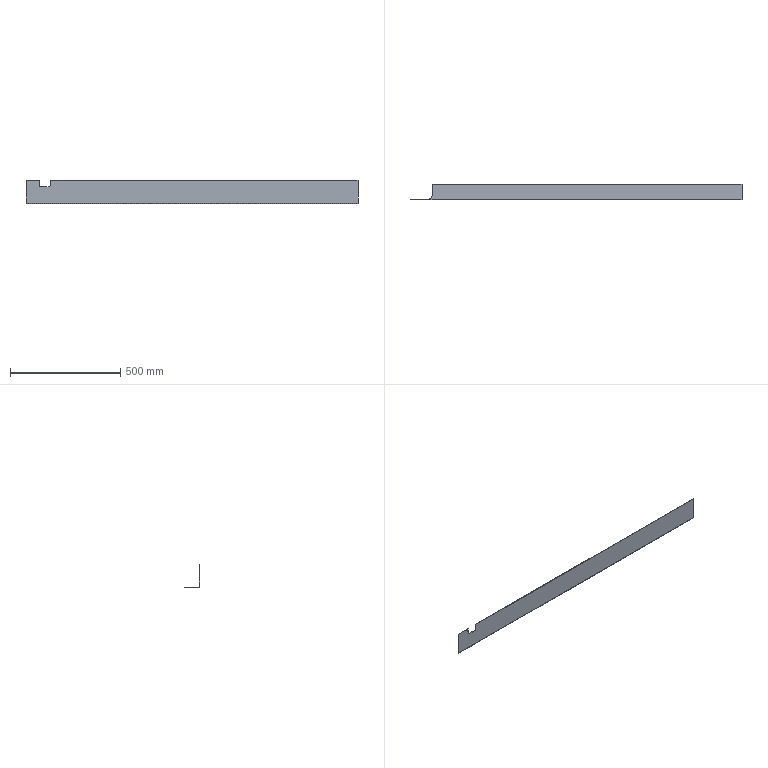Part | STEP file | Trunking 1 | 1 solid | 19 faces | box 1504 x 70 x 106 mm | volume 380057 mm3 | plane 14 | cylinder 5 | commonest cylinder face diameters 20 x2 1 x1 4 x1 40 x1
STEP:
#1=CARTESIAN_POINT('',(60.,-47.697,34.079));
#2=VERTEX_POINT('',#1);
#3=CARTESIAN_POINT('',(60.,-47.697,14.079));
#4=VERTEX_POINT('',#3);
#5=CARTESIAN_POINT('',(60.,-47.697,34.079));
#6=DIRECTION('',(0.,0.,-1.));
#7=VECTOR('',#6,1000.);
#8=LINE('',#5,#7);
#9=EDGE_CURVE('',#2,#4,#8,.T.);
#10=ORIENTED_EDGE('',*,*,#9,.F.);
#11=CARTESIAN_POINT('',(0.,-47.697,34.079));
#12=VERTEX_POINT('',#11);
#13=CARTESIAN_POINT('',(1504.,-47.697,34.079));
#14=DIRECTION('',(1.,0.,0.));
#15=VECTOR('',#14,1000.);
#16=LINE('',#13,#15);
#17=EDGE_CURVE('',#12,#2,#16,.T.);
#18=ORIENTED_EDGE('',*,*,#17,.F.);
#19=CARTESIAN_POINT('',(0.,-47.697,-69.921));
#20=VERTEX_POINT('',#19);
#21=CARTESIAN_POINT('',(0.,-47.697,34.079));
#22=DIRECTION('',(0.,0.,1.));
#23=VECTOR('',#22,1000.);
#24=LINE('',#21,#23);
#25=EDGE_CURVE('',#20,#12,#24,.T.);
#26=ORIENTED_EDGE('',*,*,#25,.F.);
#27=CARTESIAN_POINT('',(1504.,-47.697,-69.921));
#28=VERTEX_POINT('',#27);
#29=CARTESIAN_POINT('',(1504.,-47.697,-69.921));
#30=DIRECTION('',(-1.,0.,0.));
#31=VECTOR('',#30,1000.);
#32=LINE('',#29,#31);
#33=EDGE_CURVE('',#28,#20,#32,.T.);
#34=ORIENTED_EDGE('',*,*,#33,.F.);
#35=CARTESIAN_POINT('',(1504.,-47.697,34.079));
#36=VERTEX_POINT('',#35);
#37=CARTESIAN_POINT('',(1504.,-47.697,34.079));
#38=DIRECTION('',(0.,0.,-1.));
#39=VECTOR('',#38,1000.);
#40=LINE('',#37,#39);
#41=EDGE_CURVE('',#36,#28,#40,.T.);
#42=ORIENTED_EDGE('',*,*,#41,.F.);
#43=CARTESIAN_POINT('',(110.,-47.697,34.079));
#44=VERTEX_POINT('',#43);
#45=CARTESIAN_POINT('',(1504.,-47.697,34.079));
#46=DIRECTION('',(1.,0.,0.));
#47=VECTOR('',#46,1000.);
#48=LINE('',#45,#47);
#49=EDGE_CURVE('',#44,#36,#48,.T.);
#50=ORIENTED_EDGE('',*,*,#49,.F.);
#51=CARTESIAN_POINT('',(110.,-47.697,14.079));
#52=VERTEX_POINT('',#51);
#53=CARTESIAN_POINT('',(110.,-47.697,34.079));
#54=DIRECTION('',(0.,0.,1.));
#55=VECTOR('',#54,1000.);
#56=LINE('',#53,#55);
#57=EDGE_CURVE('',#52,#44,#56,.T.);
#58=ORIENTED_EDGE('',*,*,#57,.F.);
#59=CARTESIAN_POINT('',(100.,-47.697,4.079));
#60=VERTEX_POINT('',#59);
#61=CARTESIAN_POINT('',(100.,-47.697,14.079));
#62=DIRECTION('',(0.,-1.,0.));
#63=DIRECTION('',(0.,0.,1.));
#64=AXIS2_PLACEMENT_3D('',#61,#62,#63);
#65=CIRCLE('',#64,10.);
#66=EDGE_CURVE('',#60,#52,#65,.T.);
#67=ORIENTED_EDGE('',*,*,#66,.F.);
#68=CARTESIAN_POINT('',(70.,-47.697,4.079));
#69=VERTEX_POINT('',#68);
#70=CARTESIAN_POINT('',(1504.,-47.697,4.079));
#71=DIRECTION('',(1.,0.,0.));
#72=VECTOR('',#71,1000.);
#73=LINE('',#70,#72);
#74=EDGE_CURVE('',#69,#60,#73,.T.);
#75=ORIENTED_EDGE('',*,*,#74,.F.);
#76=CARTESIAN_POINT('',(70.,-47.697,14.079));
#77=DIRECTION('',(0.,-1.,0.));
#78=DIRECTION('',(0.,0.,1.));
#79=AXIS2_PLACEMENT_3D('',#76,#77,#78);
#80=CIRCLE('',#79,10.);
#81=EDGE_CURVE('',#4,#69,#80,.T.);
#82=ORIENTED_EDGE('',*,*,#81,.F.);
#83=EDGE_LOOP('',(#10,#18,#26,#34,#42,#50,#58,#67,#75,#82));
#84=FACE_OUTER_BOUND('',#83,.T.);
#85=CARTESIAN_POINT('',(1504.,-47.697,34.079));
#86=DIRECTION('',(0.,1.,0.));
#87=DIRECTION('',(0.,0.,1.));
#88=AXIS2_PLACEMENT_3D('',#85,#86,#87);
#89=PLANE('',#88);
#90=ADVANCED_FACE('',(#84),#89,.F.);
#91=CARTESIAN_POINT('',(60.,-46.197,14.079));
#92=VERTEX_POINT('',#91);
#93=CARTESIAN_POINT('',(70.,-46.197,4.079));
#94=VERTEX_POINT('',#93);
#95=CARTESIAN_POINT('',(70.,-46.197,14.079));
#96=DIRECTION('',(0.,-1.,0.));
#97=DIRECTION('',(0.,0.,1.));
#98=AXIS2_PLACEMENT_3D('',#95,#96,#97);
#99=CIRCLE('',#98,10.);
#100=EDGE_CURVE('',#92,#94,#99,.T.);
#101=ORIENTED_EDGE('',*,*,#100,.F.);
#102=CARTESIAN_POINT('',(60.,-48.197,14.079));
#103=DIRECTION('',(0.,1.,0.));
#104=VECTOR('',#103,1000.);
#105=LINE('',#102,#104);
#106=EDGE_CURVE('',#4,#92,#105,.T.);
#107=ORIENTED_EDGE('',*,*,#106,.F.);
#108=ORIENTED_EDGE('',*,*,#81,.T.);
#109=CARTESIAN_POINT('',(70.,-48.197,4.079));
#110=DIRECTION('',(0.,-1.,0.));
#111=VECTOR('',#110,1000.);
#112=LINE('',#109,#111);
#113=EDGE_CURVE('',#94,#69,#112,.T.);
#114=ORIENTED_EDGE('',*,*,#113,.F.);
#115=EDGE_LOOP('',(#101,#107,#108,#114));
#116=FACE_OUTER_BOUND('',#115,.T.);
#117=CARTESIAN_POINT('',(70.,-48.197,14.079));
#118=DIRECTION('',(0.,1.,0.));
#119=DIRECTION('',(0.,0.,1.));
#120=AXIS2_PLACEMENT_3D('',#117,#118,#119);
#121=CYLINDRICAL_SURFACE('',#120,10.);
#122=ADVANCED_FACE('',(#116),#121,.F.);
#123=CARTESIAN_POINT('',(60.,-46.197,34.079));
#124=VERTEX_POINT('',#123);
#125=CARTESIAN_POINT('',(60.,-46.197,34.079));
#126=DIRECTION('',(0.,0.,-1.));
#127=VECTOR('',#126,1000.);
#128=LINE('',#125,#127);
#129=EDGE_CURVE('',#124,#92,#128,.T.);
#130=ORIENTED_EDGE('',*,*,#129,.F.);
#131=CARTESIAN_POINT('',(60.,-48.197,34.079));
#132=DIRECTION('',(0.,1.,0.));
#133=VECTOR('',#132,1000.);
#134=LINE('',#131,#133);
#135=EDGE_CURVE('',#2,#124,#134,.T.);
#136=ORIENTED_EDGE('',*,*,#135,.F.);
#137=ORIENTED_EDGE('',*,*,#9,.T.);
#138=ORIENTED_EDGE('',*,*,#106,.T.);
#139=EDGE_LOOP('',(#130,#136,#137,#138));
#140=FACE_OUTER_BOUND('',#139,.T.);
#141=CARTESIAN_POINT('',(60.,-48.197,34.079));
#142=DIRECTION('',(-1.,0.,0.));
#143=DIRECTION('',(0.,0.,1.));
#144=AXIS2_PLACEMENT_3D('',#141,#142,#143);
#145=PLANE('',#144);
#146=ADVANCED_FACE('',(#140),#145,.F.);
#147=CARTESIAN_POINT('',(0.,-46.197,34.079));
#148=VERTEX_POINT('',#147);
#149=CARTESIAN_POINT('',(0.,-47.697,34.079));
#150=DIRECTION('',(0.,-1.,0.));
#151=VECTOR('',#150,1000.);
#152=LINE('',#149,#151);
#153=EDGE_CURVE('',#148,#12,#152,.T.);
#154=ORIENTED_EDGE('',*,*,#153,.T.);
#155=ORIENTED_EDGE('',*,*,#17,.T.);
#156=ORIENTED_EDGE('',*,*,#135,.T.);
#157=CARTESIAN_POINT('',(1504.,-46.197,34.079));
#158=DIRECTION('',(-1.,0.,0.));
#159=VECTOR('',#158,1000.);
#160=LINE('',#157,#159);
#161=EDGE_CURVE('',#124,#148,#160,.T.);
#162=ORIENTED_EDGE('',*,*,#161,.T.);
#163=EDGE_LOOP('',(#154,#155,#156,#162));
#164=FACE_OUTER_BOUND('',#163,.T.);
#165=CARTESIAN_POINT('',(1504.,-47.697,34.079));
#166=DIRECTION('',(0.,0.,1.));
#167=DIRECTION('',(1.,0.,0.));
#168=AXIS2_PLACEMENT_3D('',#165,#166,#167);
#169=PLANE('',#168);
#170=ADVANCED_FACE('',(#164),#169,.T.);
#171=CARTESIAN_POINT('',(0.,-46.197,-69.921));
#172=VERTEX_POINT('',#171);
#173=CARTESIAN_POINT('',(0.,-46.197,-69.921));
#174=DIRECTION('',(0.,0.,1.));
#175=VECTOR('',#174,1000.);
#176=LINE('',#173,#175);
#177=EDGE_CURVE('',#172,#148,#176,.T.);
#178=ORIENTED_EDGE('',*,*,#177,.F.);
#179=CARTESIAN_POINT('',(0.,-45.997,-70.321));
#180=VERTEX_POINT('',#179);
#181=CARTESIAN_POINT('',(0.,-45.697,-69.921));
#182=DIRECTION('',(1.,0.,0.));
#183=DIRECTION('',(0.,0.,1.));
#184=AXIS2_PLACEMENT_3D('',#181,#182,#183);
#185=CIRCLE('',#184,0.5);
#186=EDGE_CURVE('',#172,#180,#185,.T.);
#187=ORIENTED_EDGE('',*,*,#186,.T.);
#188=CARTESIAN_POINT('',(0.,-45.997,-71.898));
#189=VERTEX_POINT('',#188);
#190=CARTESIAN_POINT('',(0.,-45.997,-49.921));
#191=DIRECTION('',(0.,0.,-1.));
#192=VECTOR('',#191,1000.);
#193=LINE('',#190,#192);
#194=EDGE_CURVE('',#180,#189,#193,.T.);
#195=ORIENTED_EDGE('',*,*,#194,.T.);
#196=CARTESIAN_POINT('',(0.,-45.697,-69.921));
#197=DIRECTION('',(1.,0.,0.));
#198=DIRECTION('',(0.,0.,1.));
#199=AXIS2_PLACEMENT_3D('',#196,#197,#198);
#200=CIRCLE('',#199,2.);
#201=EDGE_CURVE('',#20,#189,#200,.T.);
#202=ORIENTED_EDGE('',*,*,#201,.F.);
#203=ORIENTED_EDGE('',*,*,#25,.T.);
#204=ORIENTED_EDGE('',*,*,#153,.F.);
#205=EDGE_LOOP('',(#178,#187,#195,#202,#203,#204));
#206=FACE_OUTER_BOUND('',#205,.T.);
#207=CARTESIAN_POINT('',(0.,-45.697,-69.921));
#208=DIRECTION('',(1.,0.,0.));
#209=DIRECTION('',(0.,0.,-1.));
#210=AXIS2_PLACEMENT_3D('',#207,#208,#209);
#211=PLANE('',#210);
#212=ADVANCED_FACE('',(#206),#211,.F.);
#213=CARTESIAN_POINT('',(1504.,-45.697,-71.921));
#214=VERTEX_POINT('',#213);
#215=CARTESIAN_POINT('',(1504.,-45.697,-69.921));
#216=DIRECTION('',(-1.,0.,0.));
#217=DIRECTION('',(0.,0.,1.));
#218=AXIS2_PLACEMENT_3D('',#215,#216,#217);
#219=CIRCLE('',#218,2.);
#220=EDGE_CURVE('',#214,#28,#219,.T.);
#221=ORIENTED_EDGE('',*,*,#220,.T.);
#222=ORIENTED_EDGE('',*,*,#33,.T.);
#223=ORIENTED_EDGE('',*,*,#201,.T.);
#224=CARTESIAN_POINT('',(81.,-45.997,-71.898));
#225=VERTEX_POINT('',#224);
#226=CARTESIAN_POINT('',(1504.,-45.997,-71.898));
#227=DIRECTION('',(1.,0.,0.));
#228=VECTOR('',#227,1000.);
#229=LINE('',#226,#228);
#230=EDGE_CURVE('',#189,#225,#229,.T.);
#231=ORIENTED_EDGE('',*,*,#230,.T.);
#232=CARTESIAN_POINT('',(84.451,-45.697,-71.921));
#233=VERTEX_POINT('',#232);
#234=CARTESIAN_POINT('',(81.,-45.997,-71.898));
#235=CARTESIAN_POINT('',(81.58,-45.997,-71.898));
#236=CARTESIAN_POINT('',(82.157,-45.972,-71.903));
#237=CARTESIAN_POINT('',(83.307,-45.872,-71.914));
#238=CARTESIAN_POINT('',(83.88,-45.797,-71.921));
#239=CARTESIAN_POINT('',(84.451,-45.697,-71.921));
#240=B_SPLINE_CURVE_WITH_KNOTS('',3,(#234,#235,#236,#237,#238,#239),.UNSPECIFIED.,.F.,.F.,(4,2,4),(0.,0.001732,0.003464),.UNSPECIFIED.);
#241=EDGE_CURVE('',#225,#233,#240,.T.);
#242=ORIENTED_EDGE('',*,*,#241,.T.);
#243=CARTESIAN_POINT('',(1504.,-45.697,-71.921));
#244=DIRECTION('',(1.,0.,0.));
#245=VECTOR('',#244,1000.);
#246=LINE('',#243,#245);
#247=EDGE_CURVE('',#233,#214,#246,.T.);
#248=ORIENTED_EDGE('',*,*,#247,.T.);
#249=EDGE_LOOP('',(#221,#222,#223,#231,#242,#248));
#250=FACE_OUTER_BOUND('',#249,.T.);
#251=CARTESIAN_POINT('',(1504.,-45.697,-69.921));
#252=DIRECTION('',(-1.,0.,0.));
#253=DIRECTION('',(0.,0.,1.));
#254=AXIS2_PLACEMENT_3D('',#251,#252,#253);
#255=CYLINDRICAL_SURFACE('',#254,2.);
#256=ADVANCED_FACE('',(#250),#255,.T.);
#257=CARTESIAN_POINT('',(1504.,-46.197,-69.921));
#258=VERTEX_POINT('',#257);
#259=CARTESIAN_POINT('',(1504.,-46.197,34.079));
#260=VERTEX_POINT('',#259);
#261=CARTESIAN_POINT('',(1504.,-46.197,-70.421));
#262=DIRECTION('',(0.,0.,1.));
#263=VECTOR('',#262,1000.);
#264=LINE('',#261,#263);
#265=EDGE_CURVE('',#258,#260,#264,.T.);
#266=ORIENTED_EDGE('',*,*,#265,.T.);
#267=CARTESIAN_POINT('',(1504.,-45.697,34.079));
#268=DIRECTION('',(0.,-1.,0.));
#269=VECTOR('',#268,1000.);
#270=LINE('',#267,#269);
#271=EDGE_CURVE('',#260,#36,#270,.T.);
#272=ORIENTED_EDGE('',*,*,#271,.T.);
#273=ORIENTED_EDGE('',*,*,#41,.T.);
#274=ORIENTED_EDGE('',*,*,#220,.F.);
#275=CARTESIAN_POINT('',(1504.,22.303,-71.921));
#276=VERTEX_POINT('',#275);
#277=CARTESIAN_POINT('',(1504.,-47.697,-71.921));
#278=DIRECTION('',(0.,1.,0.));
#279=VECTOR('',#278,1000.);
#280=LINE('',#277,#279);
#281=EDGE_CURVE('',#214,#276,#280,.T.);
#282=ORIENTED_EDGE('',*,*,#281,.T.);
#283=CARTESIAN_POINT('',(1504.,22.303,-70.421));
#284=VERTEX_POINT('',#283);
#285=CARTESIAN_POINT('',(1504.,22.303,-70.421));
#286=DIRECTION('',(0.,0.,-1.));
#287=VECTOR('',#286,1000.);
#288=LINE('',#285,#287);
#289=EDGE_CURVE('',#284,#276,#288,.T.);
#290=ORIENTED_EDGE('',*,*,#289,.F.);
#291=CARTESIAN_POINT('',(1504.,-45.697,-70.421));
#292=VERTEX_POINT('',#291);
#293=CARTESIAN_POINT('',(1504.,-45.697,-70.421));
#294=DIRECTION('',(0.,-1.,0.));
#295=VECTOR('',#294,1000.);
#296=LINE('',#293,#295);
#297=EDGE_CURVE('',#284,#292,#296,.T.);
#298=ORIENTED_EDGE('',*,*,#297,.T.);
#299=CARTESIAN_POINT('',(1504.,-45.697,-69.921));
#300=DIRECTION('',(-1.,0.,0.));
#301=DIRECTION('',(0.,0.,1.));
#302=AXIS2_PLACEMENT_3D('',#299,#300,#301);
#303=CIRCLE('',#302,0.5);
#304=EDGE_CURVE('',#292,#258,#303,.T.);
#305=ORIENTED_EDGE('',*,*,#304,.T.);
#306=EDGE_LOOP('',(#266,#272,#273,#274,#282,#290,#298,#305));
#307=FACE_OUTER_BOUND('',#306,.T.);
#308=CARTESIAN_POINT('',(1504.,-45.697,-70.421));
#309=DIRECTION('',(1.,0.,0.));
#310=DIRECTION('',(0.,0.,-1.));
#311=AXIS2_PLACEMENT_3D('',#308,#309,#310);
#312=PLANE('',#311);
#313=ADVANCED_FACE('',(#307),#312,.T.);
#314=ORIENTED_EDGE('',*,*,#271,.F.);
#315=CARTESIAN_POINT('',(110.,-46.197,34.079));
#316=VERTEX_POINT('',#315);
#317=CARTESIAN_POINT('',(1504.,-46.197,34.079));
#318=DIRECTION('',(-1.,0.,0.));
#319=VECTOR('',#318,1000.);
#320=LINE('',#317,#319);
#321=EDGE_CURVE('',#260,#316,#320,.T.);
#322=ORIENTED_EDGE('',*,*,#321,.T.);
#323=CARTESIAN_POINT('',(110.,-47.697,34.079));
#324=DIRECTION('',(0.,-1.,0.));
#325=VECTOR('',#324,1000.);
#326=LINE('',#323,#325);
#327=EDGE_CURVE('',#316,#44,#326,.T.);
#328=ORIENTED_EDGE('',*,*,#327,.T.);
#329=ORIENTED_EDGE('',*,*,#49,.T.);
#330=EDGE_LOOP('',(#314,#322,#328,#329));
#331=FACE_OUTER_BOUND('',#330,.T.);
#332=CARTESIAN_POINT('',(1504.,-47.697,34.079));
#333=DIRECTION('',(0.,0.,1.));
#334=DIRECTION('',(1.,0.,0.));
#335=AXIS2_PLACEMENT_3D('',#332,#333,#334);
#336=PLANE('',#335);
#337=ADVANCED_FACE('',(#331),#336,.T.);
#338=CARTESIAN_POINT('',(110.,-46.197,14.079));
#339=VERTEX_POINT('',#338);
#340=CARTESIAN_POINT('',(110.,-46.197,34.079));
#341=DIRECTION('',(0.,0.,1.));
#342=VECTOR('',#341,1000.);
#343=LINE('',#340,#342);
#344=EDGE_CURVE('',#339,#316,#343,.T.);
#345=ORIENTED_EDGE('',*,*,#344,.F.);
#346=CARTESIAN_POINT('',(110.,-48.197,14.079));
#347=DIRECTION('',(0.,1.,0.));
#348=VECTOR('',#347,1000.);
#349=LINE('',#346,#348);
#350=EDGE_CURVE('',#52,#339,#349,.T.);
#351=ORIENTED_EDGE('',*,*,#350,.F.);
#352=ORIENTED_EDGE('',*,*,#57,.T.);
#353=ORIENTED_EDGE('',*,*,#327,.F.);
#354=EDGE_LOOP('',(#345,#351,#352,#353));
#355=FACE_OUTER_BOUND('',#354,.T.);
#356=CARTESIAN_POINT('',(110.,-48.197,34.079));
#357=DIRECTION('',(1.,0.,0.));
#358=DIRECTION('',(0.,0.,-1.));
#359=AXIS2_PLACEMENT_3D('',#356,#357,#358);
#360=PLANE('',#359);
#361=ADVANCED_FACE('',(#355),#360,.F.);
#362=CARTESIAN_POINT('',(100.,-46.197,4.079));
#363=VERTEX_POINT('',#362);
#364=CARTESIAN_POINT('',(100.,-46.197,14.079));
#365=DIRECTION('',(0.,-1.,0.));
#366=DIRECTION('',(0.,0.,1.));
#367=AXIS2_PLACEMENT_3D('',#364,#365,#366);
#368=CIRCLE('',#367,10.);
#369=EDGE_CURVE('',#363,#339,#368,.T.);
#370=ORIENTED_EDGE('',*,*,#369,.F.);
#371=CARTESIAN_POINT('',(100.,-48.197,4.079));
#372=DIRECTION('',(0.,1.,0.));
#373=VECTOR('',#372,1000.);
#374=LINE('',#371,#373);
#375=EDGE_CURVE('',#60,#363,#374,.T.);
#376=ORIENTED_EDGE('',*,*,#375,.F.);
#377=ORIENTED_EDGE('',*,*,#66,.T.);
#378=ORIENTED_EDGE('',*,*,#350,.T.);
#379=EDGE_LOOP('',(#370,#376,#377,#378));
#380=FACE_OUTER_BOUND('',#379,.T.);
#381=CARTESIAN_POINT('',(100.,-48.197,14.079));
#382=DIRECTION('',(0.,1.,0.));
#383=DIRECTION('',(0.,0.,1.));
#384=AXIS2_PLACEMENT_3D('',#381,#382,#383);
#385=CYLINDRICAL_SURFACE('',#384,10.);
#386=ADVANCED_FACE('',(#380),#385,.F.);
#387=CARTESIAN_POINT('',(70.,-46.197,4.079));
#388=DIRECTION('',(1.,0.,0.));
#389=VECTOR('',#388,1000.);
#390=LINE('',#387,#389);
#391=EDGE_CURVE('',#94,#363,#390,.T.);
#392=ORIENTED_EDGE('',*,*,#391,.F.);
#393=ORIENTED_EDGE('',*,*,#113,.T.);
#394=ORIENTED_EDGE('',*,*,#74,.T.);
#395=ORIENTED_EDGE('',*,*,#375,.T.);
#396=EDGE_LOOP('',(#392,#393,#394,#395));
#397=FACE_OUTER_BOUND('',#396,.T.);
#398=CARTESIAN_POINT('',(70.,-48.197,4.079));
#399=DIRECTION('',(0.,0.,-1.));
#400=DIRECTION('',(-1.,0.,0.));
#401=AXIS2_PLACEMENT_3D('',#398,#399,#400);
#402=PLANE('',#401);
#403=ADVANCED_FACE('',(#397),#402,.F.);
#404=ORIENTED_EDGE('',*,*,#177,.T.);
#405=ORIENTED_EDGE('',*,*,#161,.F.);
#406=ORIENTED_EDGE('',*,*,#129,.T.);
#407=ORIENTED_EDGE('',*,*,#100,.T.);
#408=ORIENTED_EDGE('',*,*,#391,.T.);
#409=ORIENTED_EDGE('',*,*,#369,.T.);
#410=ORIENTED_EDGE('',*,*,#344,.T.);
#411=ORIENTED_EDGE('',*,*,#321,.F.);
#412=ORIENTED_EDGE('',*,*,#265,.F.);
#413=CARTESIAN_POINT('',(1504.,-46.197,-69.921));
#414=DIRECTION('',(-1.,0.,0.));
#415=VECTOR('',#414,1000.);
#416=LINE('',#413,#415);
#417=EDGE_CURVE('',#258,#172,#416,.T.);
#418=ORIENTED_EDGE('',*,*,#417,.T.);
#419=EDGE_LOOP('',(#404,#405,#406,#407,#408,#409,#410,#411,#412,#418));
#420=FACE_OUTER_BOUND('',#419,.T.);
#421=CARTESIAN_POINT('',(1504.,-46.197,34.079));
#422=DIRECTION('',(0.,1.,0.));
#423=DIRECTION('',(0.,0.,1.));
#424=AXIS2_PLACEMENT_3D('',#421,#422,#423);
#425=PLANE('',#424);
#426=ADVANCED_FACE('',(#420),#425,.T.);
#427=CARTESIAN_POINT('',(101.,-25.997,-71.921));
#428=VERTEX_POINT('',#427);
#429=CARTESIAN_POINT('',(81.,-25.997,-71.921));
#430=DIRECTION('',(0.,0.,-1.));
#431=DIRECTION('',(0.,1.,0.));
#432=AXIS2_PLACEMENT_3D('',#429,#430,#431);
#433=CIRCLE('',#432,20.);
#434=EDGE_CURVE('',#428,#233,#433,.T.);
#435=ORIENTED_EDGE('',*,*,#434,.F.);
#436=CARTESIAN_POINT('',(101.,22.303,-71.921));
#437=VERTEX_POINT('',#436);
#438=CARTESIAN_POINT('',(101.,-47.697,-71.921));
#439=DIRECTION('',(0.,-1.,0.));
#440=VECTOR('',#439,1000.);
#441=LINE('',#438,#440);
#442=EDGE_CURVE('',#437,#428,#441,.T.);
#443=ORIENTED_EDGE('',*,*,#442,.F.);
#444=CARTESIAN_POINT('',(1504.,22.303,-71.921));
#445=DIRECTION('',(-1.,0.,0.));
#446=VECTOR('',#445,1000.);
#447=LINE('',#444,#446);
#448=EDGE_CURVE('',#276,#437,#447,.T.);
#449=ORIENTED_EDGE('',*,*,#448,.F.);
#450=ORIENTED_EDGE('',*,*,#281,.F.);
#451=ORIENTED_EDGE('',*,*,#247,.F.);
#452=EDGE_LOOP('',(#435,#443,#449,#450,#451));
#453=FACE_OUTER_BOUND('',#452,.T.);
#454=CARTESIAN_POINT('',(1504.,-47.697,-71.921));
#455=DIRECTION('',(0.,0.,1.));
#456=DIRECTION('',(0.,-1.,0.));
#457=AXIS2_PLACEMENT_3D('',#454,#455,#456);
#458=PLANE('',#457);
#459=ADVANCED_FACE('',(#453),#458,.F.);
#460=CARTESIAN_POINT('',(101.,-25.997,-70.421));
#461=VERTEX_POINT('',#460);
#462=CARTESIAN_POINT('',(101.,-25.997,-49.921));
#463=DIRECTION('',(0.,0.,1.));
#464=VECTOR('',#463,1000.);
#465=LINE('',#462,#464);
#466=EDGE_CURVE('',#428,#461,#465,.T.);
#467=ORIENTED_EDGE('',*,*,#466,.F.);
#468=ORIENTED_EDGE('',*,*,#434,.T.);
#469=ORIENTED_EDGE('',*,*,#241,.F.);
#470=CARTESIAN_POINT('',(81.,-45.997,-70.321));
#471=VERTEX_POINT('',#470);
#472=CARTESIAN_POINT('',(81.,-45.997,-49.921));
#473=DIRECTION('',(0.,0.,-1.));
#474=VECTOR('',#473,1000.);
#475=LINE('',#472,#474);
#476=EDGE_CURVE('',#471,#225,#475,.T.);
#477=ORIENTED_EDGE('',*,*,#476,.F.);
#478=CARTESIAN_POINT('',(84.451,-45.697,-70.421));
#479=VERTEX_POINT('',#478);
#480=CARTESIAN_POINT('',(84.451,-45.697,-70.421));
#481=CARTESIAN_POINT('',(83.881,-45.797,-70.421));
#482=CARTESIAN_POINT('',(83.307,-45.872,-70.393));
#483=CARTESIAN_POINT('',(82.156,-45.972,-70.342));
#484=CARTESIAN_POINT('',(81.579,-45.997,-70.321));
#485=CARTESIAN_POINT('',(81.,-45.997,-70.321));
#486=B_SPLINE_CURVE_WITH_KNOTS('',3,(#480,#481,#482,#483,#484,#485),.UNSPECIFIED.,.F.,.F.,(4,2,4),(0.,0.001736,0.003472),.UNSPECIFIED.);
#487=EDGE_CURVE('',#479,#471,#486,.T.);
#488=ORIENTED_EDGE('',*,*,#487,.F.);
#489=CARTESIAN_POINT('',(81.,-25.997,-70.421));
#490=DIRECTION('',(0.,0.,-1.));
#491=DIRECTION('',(0.,1.,0.));
#492=AXIS2_PLACEMENT_3D('',#489,#490,#491);
#493=CIRCLE('',#492,20.);
#494=EDGE_CURVE('',#461,#479,#493,.T.);
#495=ORIENTED_EDGE('',*,*,#494,.F.);
#496=EDGE_LOOP('',(#467,#468,#469,#477,#488,#495));
#497=FACE_OUTER_BOUND('',#496,.T.);
#498=CARTESIAN_POINT('',(81.,-25.997,-49.921));
#499=DIRECTION('',(0.,0.,-1.));
#500=DIRECTION('',(0.,1.,0.));
#501=AXIS2_PLACEMENT_3D('',#498,#499,#500);
#502=CYLINDRICAL_SURFACE('',#501,20.);
#503=ADVANCED_FACE('',(#497),#502,.F.);
#504=ORIENTED_EDGE('',*,*,#476,.T.);
#505=ORIENTED_EDGE('',*,*,#230,.F.);
#506=ORIENTED_EDGE('',*,*,#194,.F.);
#507=CARTESIAN_POINT('',(0.,-45.997,-70.321));
#508=DIRECTION('',(-1.,0.,0.));
#509=VECTOR('',#508,1000.);
#510=LINE('',#507,#509);
#511=EDGE_CURVE('',#471,#180,#510,.T.);
#512=ORIENTED_EDGE('',*,*,#511,.F.);
#513=EDGE_LOOP('',(#504,#505,#506,#512));
#514=FACE_OUTER_BOUND('',#513,.T.);
#515=CARTESIAN_POINT('',(0.,-45.997,-49.921));
#516=DIRECTION('',(0.,-1.,0.));
#517=DIRECTION('',(0.,0.,-1.));
#518=AXIS2_PLACEMENT_3D('',#515,#516,#517);
#519=PLANE('',#518);
#520=ADVANCED_FACE('',(#514),#519,.F.);
#521=ORIENTED_EDGE('',*,*,#186,.F.);
#522=ORIENTED_EDGE('',*,*,#417,.F.);
#523=ORIENTED_EDGE('',*,*,#304,.F.);
#524=CARTESIAN_POINT('',(1504.,-45.697,-70.421));
#525=DIRECTION('',(1.,0.,0.));
#526=VECTOR('',#525,1000.);
#527=LINE('',#524,#526);
#528=EDGE_CURVE('',#479,#292,#527,.T.);
#529=ORIENTED_EDGE('',*,*,#528,.F.);
#530=ORIENTED_EDGE('',*,*,#487,.T.);
#531=ORIENTED_EDGE('',*,*,#511,.T.);
#532=EDGE_LOOP('',(#521,#522,#523,#529,#530,#531));
#533=FACE_OUTER_BOUND('',#532,.T.);
#534=CARTESIAN_POINT('',(1504.,-45.697,-69.921));
#535=DIRECTION('',(-1.,0.,0.));
#536=DIRECTION('',(0.,0.,1.));
#537=AXIS2_PLACEMENT_3D('',#534,#535,#536);
#538=CYLINDRICAL_SURFACE('',#537,0.5);
#539=ADVANCED_FACE('',(#533),#538,.F.);
#540=CARTESIAN_POINT('',(101.,22.303,-70.421));
#541=VERTEX_POINT('',#540);
#542=CARTESIAN_POINT('',(101.,22.303,-49.921));
#543=DIRECTION('',(0.,0.,1.));
#544=VECTOR('',#543,1000.);
#545=LINE('',#542,#544);
#546=EDGE_CURVE('',#437,#541,#545,.T.);
#547=ORIENTED_EDGE('',*,*,#546,.F.);
#548=ORIENTED_EDGE('',*,*,#442,.T.);
#549=ORIENTED_EDGE('',*,*,#466,.T.);
#550=CARTESIAN_POINT('',(101.,22.303,-70.421));
#551=DIRECTION('',(0.,-1.,0.));
#552=VECTOR('',#551,1000.);
#553=LINE('',#550,#552);
#554=EDGE_CURVE('',#541,#461,#553,.T.);
#555=ORIENTED_EDGE('',*,*,#554,.F.);
#556=EDGE_LOOP('',(#547,#548,#549,#555));
#557=FACE_OUTER_BOUND('',#556,.T.);
#558=CARTESIAN_POINT('',(101.,22.303,-49.921));
#559=DIRECTION('',(1.,0.,0.));
#560=DIRECTION('',(0.,0.,-1.));
#561=AXIS2_PLACEMENT_3D('',#558,#559,#560);
#562=PLANE('',#561);
#563=ADVANCED_FACE('',(#557),#562,.F.);
#564=ORIENTED_EDGE('',*,*,#289,.T.);
#565=ORIENTED_EDGE('',*,*,#448,.T.);
#566=ORIENTED_EDGE('',*,*,#546,.T.);
#567=CARTESIAN_POINT('',(1504.,22.303,-70.421));
#568=DIRECTION('',(1.,0.,0.));
#569=VECTOR('',#568,1000.);
#570=LINE('',#567,#569);
#571=EDGE_CURVE('',#541,#284,#570,.T.);
#572=ORIENTED_EDGE('',*,*,#571,.T.);
#573=EDGE_LOOP('',(#564,#565,#566,#572));
#574=FACE_OUTER_BOUND('',#573,.T.);
#575=CARTESIAN_POINT('',(1504.,22.303,-70.421));
#576=DIRECTION('',(0.,1.,0.));
#577=DIRECTION('',(0.,0.,1.));
#578=AXIS2_PLACEMENT_3D('',#575,#576,#577);
#579=PLANE('',#578);
#580=ADVANCED_FACE('',(#574),#579,.T.);
#581=ORIENTED_EDGE('',*,*,#571,.F.);
#582=ORIENTED_EDGE('',*,*,#554,.T.);
#583=ORIENTED_EDGE('',*,*,#494,.T.);
#584=ORIENTED_EDGE('',*,*,#528,.T.);
#585=ORIENTED_EDGE('',*,*,#297,.F.);
#586=EDGE_LOOP('',(#581,#582,#583,#584,#585));
#587=FACE_OUTER_BOUND('',#586,.T.);
#588=CARTESIAN_POINT('',(1504.,-47.697,-70.421));
#589=DIRECTION('',(0.,0.,1.));
#590=DIRECTION('',(0.,-1.,0.));
#591=AXIS2_PLACEMENT_3D('',#588,#589,#590);
#592=PLANE('',#591);
#593=ADVANCED_FACE('',(#587),#592,.T.);
#594=CLOSED_SHELL('',(#90,#122,#146,#170,#212,#256,#313,#337,#361,#386,#403,#426,#459,#503,#520,#539,#563,#580,#593));
#595=MANIFOLD_SOLID_BREP('',#594);
#596=CARTESIAN_POINT('',(0.,0.,0.));
#597=DIRECTION('',(0.,0.,1.));
#598=DIRECTION('',(1.,0.,0.));
#599=AXIS2_PLACEMENT_3D('',#596,#597,#598);
#600=(LENGTH_UNIT()NAMED_UNIT(*)SI_UNIT(.MILLI.,.METRE.));
#601=UNCERTAINTY_MEASURE_WITH_UNIT(LENGTH_MEASURE(0.00001),#600,'','');
#602=(NAMED_UNIT(*)PLANE_ANGLE_UNIT()SI_UNIT($,.RADIAN.));
#603=(NAMED_UNIT(*)SI_UNIT($,.STERADIAN.)SOLID_ANGLE_UNIT());
#604=(GEOMETRIC_REPRESENTATION_CONTEXT(3)GLOBAL_UNCERTAINTY_ASSIGNED_CONTEXT((#601))GLOBAL_UNIT_ASSIGNED_CONTEXT((#600,#602,#603))REPRESENTATION_CONTEXT('',''));
#605=ADVANCED_BREP_SHAPE_REPRESENTATION('',(#595,#599),#604);